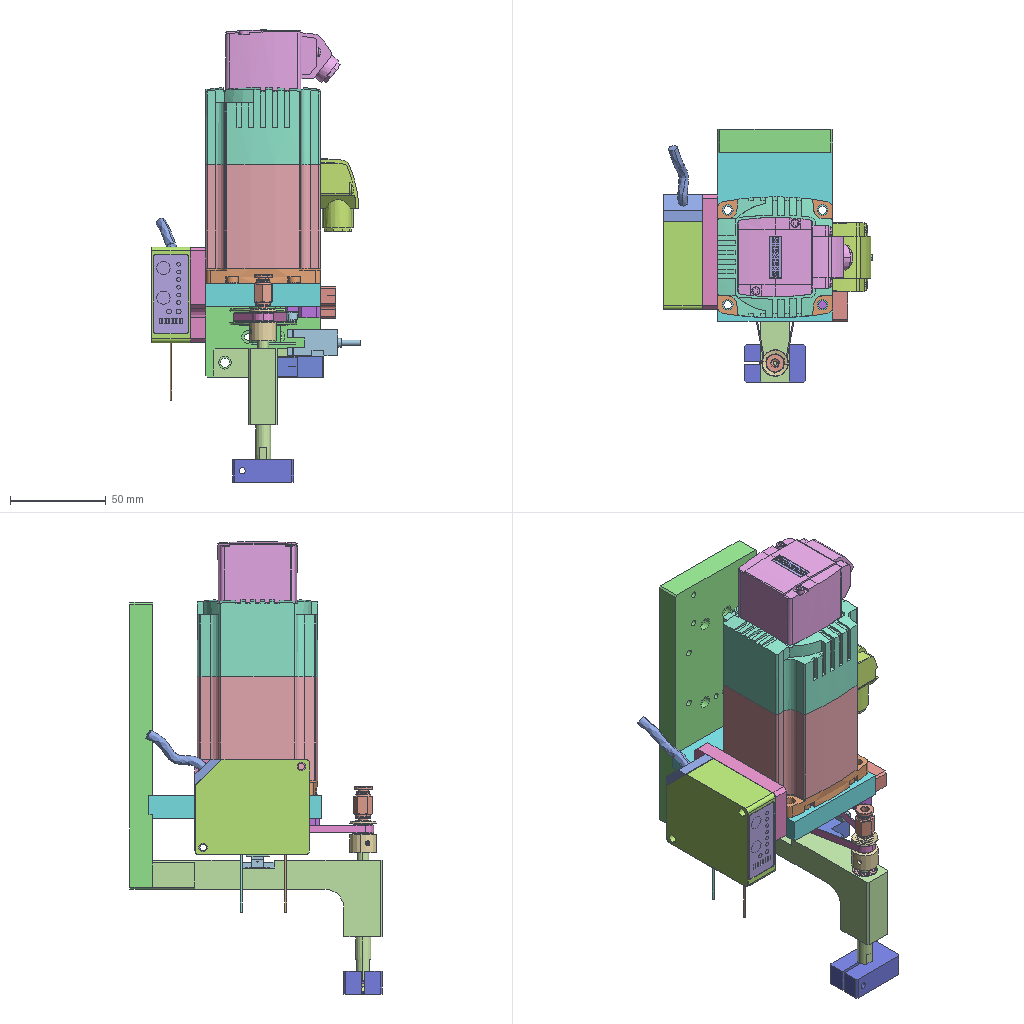Assembly | SolidWorks | 30 different items | 33 placed | box 109 x 132 x 237 mm
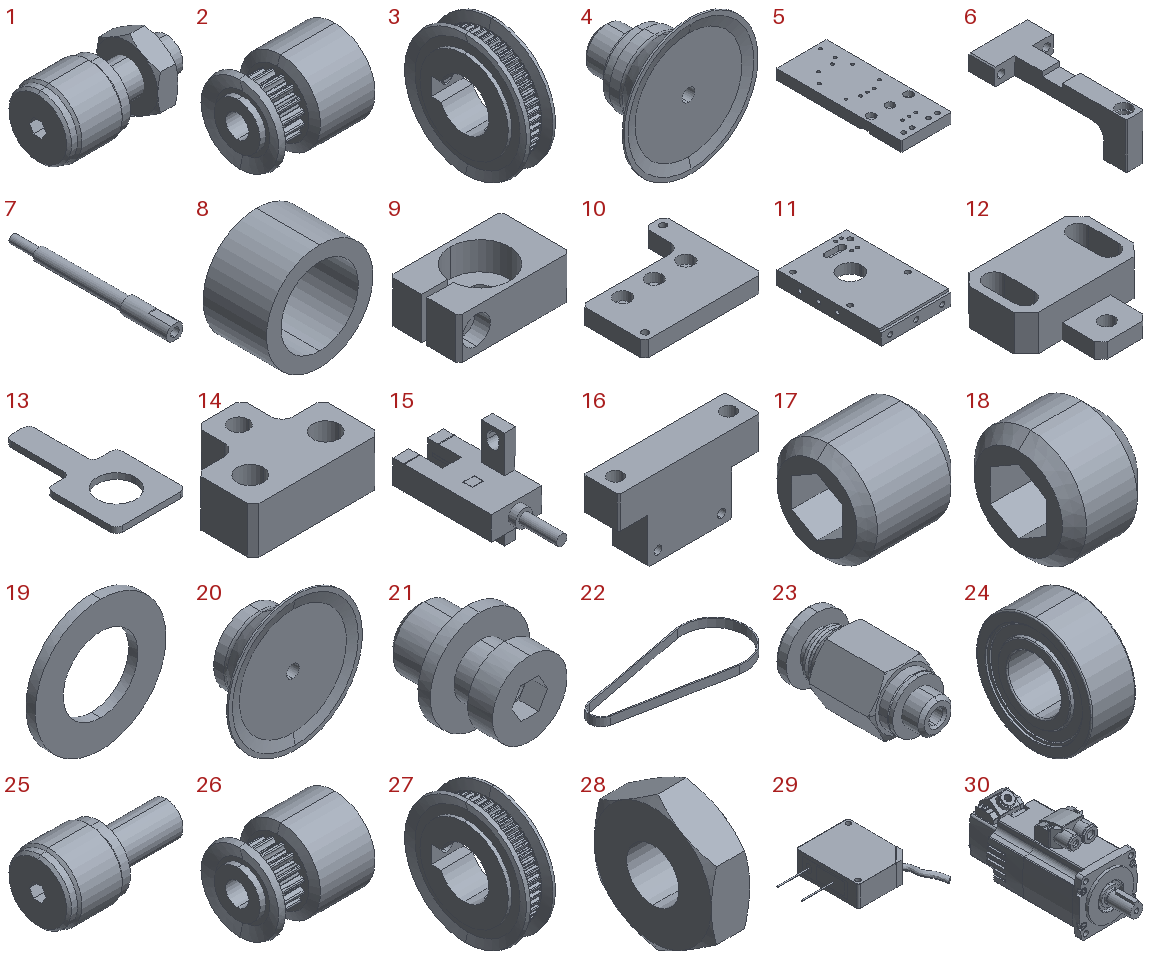Parts list (item | name | quantity | parent item | size | volume | features):
1 | (subassembly) | x1 | - | 11.5 x 6 x 6.351 mm | 226.743 mm3 | -
2 | (subassembly) | x1 | - | 17 x 14 x 14 mm | 1805 mm3 | -
3 | (subassembly) | x1 | - | 9 x 35 x 35 mm | 4712 mm3 | -
4 | (subassembly) | x1 | - | 16 x 10.5 x 16 mm | 558.242 mm3 | features AEMSimFeature 1
5 | - | x1 | - | 60 x 150 x 12 mm | 102302 mm3 | features HoleWzd 8, ICE 2, Chamfer 1, Extrusion 1, LPattern 1
6 | - | x1 | - | 52 x 120 x 40 mm | 40575 mm3 | features ICE 10, HoleWzd 3, Chamfer 1, Extrusion 1, Fillet 1, MirrorPattern 1
7 | - | x1 | - | 8 x 80 x 8 mm | 2165 mm3 | features ICE 4, HoleWzd 1, Revolution 1
8 | - | x1 | - | 8.4 x 5 x 8.4 mm | 130.965 mm3 | features Revolution 1
9 | - | x1 | - | 32 x 20 x 12 mm | 5110 mm3 | features ICE 3, HoleWzd 2, Chamfer 1, Extrusion 1, RevCut 1
10 | - | x1 | - | 60 x 50 x 8 mm | 15791 mm3 | features Chamfer 2, HoleWzd 2, Extrusion 1, Fillet 1, ICE 1
11 | - | x1 | - | 60 x 90 x 12 mm | 52743 mm3 | features HoleWzd 7, ICE 5, Chamfer 1, Cut 1, Extrusion 1, MoveFace 1
12 | - | x1 | - | 20 x 18 x 6 mm | 1134 mm3 | features HoleWzd 3, Chamfer 2, ICE 2, Extrusion 1
13 | - | x1 | - | 12 x 23 x 1 mm | 152.93 mm3 | features Extrusion 1, Fillet 1, HoleWzd 1
14 | - | x1 | - | 22 x 17 x 8 mm | 1559 mm3 | features HoleWzd 2, Chamfer 1, Extrusion 1, Fillet 1, ICE 1
15 | - | x1 | - | 13.7 x 38.4 x 26 mm | 2302 mm3 | features BaseBody 1
16 | - | x1 | - | 44 x 11 x 24 mm | 8094 mm3 | features Chamfer 2, HoleWzd 2, Extrusion 1, ICE 1
17 | - | x2 | in 2 | 3 x 3 x 3 mm | 17.153 mm3 | features BaseBody 1
18 | - | x2 | in 3 | 3 x 4 x 4 mm | 27.73 mm3 | features BaseBody 1
19 | - | x1 | in 4 | 7 x 0.5 x 7 mm | 12.959 mm3 | features BaseBody 1
20 | - | x1 | in 4 | 16 x 5.5 x 16 mm | 386.03 mm3 | features BaseBody 1
21 | - | x1 | in 4 | 8 x 9 x 8 mm | 159.238 mm3 | features BaseBody 1
22 | - | x1 | - | 76.775 x 31.76 x 4 mm | 427.631 mm3 | features Extrusion 1
23 | - | x1 | - | 10.392 x 19.5 x 9.5 mm | 848.774 mm3 | features BaseBody 1
24 | - | x2 | - | 5 x 13 x 13 mm | 402.825 mm3 | features BaseBody 1
25 | - | x1 | in 1 | 11.5 x 6 x 6 mm | 188.495 mm3 | features BaseBody 1
26 | - | x1 | in 2 | 17 x 14 x 14 mm | 1770 mm3 | features BaseBody 1
27 | - | x1 | in 3 | 9 x 35 x 35 mm | 4657 mm3 | features BaseBody 1
28 | - | x1 | in 1 | 1.8 x 5.5 x 6.351 mm | 38.246 mm3 | features BaseBody 1
29 | - | x1 | - | 95.223 x 85.573 x 20.4 mm | 60474 mm3 | features BaseBody 6
30 | - | x1 | - | 63.062 x 163.688 x 80 mm | 352083 mm3 | features BaseBody 8
Mates (type | each side: item.copy, entity, surface, feature):
Concentric | 7.1 face cylinder Revolve1 | 24.1 face cylinder Input1
Coincident | 8.1 face plane Revolve1 | 24.1 face plane Input1
Coincident | 24.1 face plane Input1 | 6.1 face plane Cut-Extrude6
Concentric | 7.1 face cylinder Revolve1 | 24.2 face cylinder Input1
Coincident | 7.1 face plane Revolve1 | 24.2 face plane Input1
Coincident | 24.2 face plane Input1 | 6.1 face plane Cut-Extrude7
Coincident | 29.1 face plane Input2 | 10.1 face plane Boss-Extrude1
Concentric | 29.1 face cylinder Input2 | 10.1 face cylinder M4 Tapped Hole1 | 2 times
Coincident | 5.1 face plane Boss-Extrude1 | 6.1 face plane Boss-Extrude1 | 2 times
Width | 6.1 face plane Boss-Extrude1 | 6.1 face plane Boss-Extrude1 | 5.1 face plane Boss-Extrude1 | 5.1 face plane Boss-Extrude1 | 2 times
Coincident | 5.1 face plane Cut-Extrude2 | 11.1 face plane Boss-Extrude1
Concentric | 5.1 face cylinder CBORE for M5 Hex Socket Head Cap Screw1 | 11.1 face cylinder M5 Tapped Hole1 | 2 times
Concentric | 7.1 face cylinder Revolve1 | 8.1 face cylinder Revolve1
Coincident | 15.1 face plane Input1 | 16.1 face plane Boss-Extrude1
Slot | 15.1 face plane Input1 | 16.1 face cylinder M3 Tapped Hole1 | 2 times
Concentric | 7.1 face cylinder M5x0.75 Tapped Hole1 | 21.1 face cylinder ZP2A-M02P_MT
Coincident | 7.1 face plane Revolve1 | 19.1 face plane ZP-5G2_MT
Coincident | 9.1 face plane Boss-Extrude1 | 20.1 face plane ZP2-B15MTS_PAD
Concentric | 7.1 face cylinder Revolve1 | 9.1 edge
Parallel | 6.1 face plane Boss-Extrude1 | 9.1 face plane Boss-Extrude1
Concentric | 7.1 face cylinder Revolve1 | 6.1 face cylinder Cut-Extrude7
Width | 22.1 face plane Boss-Extrude1 | 22.1 face plane Boss-Extrude1 | 6.1 face plane Mirror1 | 6.1 face plane Cut-Extrude4
Coincident | 6.1 face plane Mirror1 | 16.1 face plane Boss-Extrude1
Coincident | 6.1 face plane Cut-Extrude8 | 16.1 face plane Boss-Extrude1
Width | 16.1 face plane Boss-Extrude1 | 16.1 face plane Boss-Extrude1 | 6.1 face plane Cut-Extrude8 | 6.1 face plane Cut-Extrude8
Coincident | 10.1 face plane Boss-Extrude1 | 11.1 face plane Boss-Extrude1
Concentric | 10.1 face cylinder CBORE for M4 Hex Socket Head Cap Screw1 | 11.1 face cylinder M4 Tapped Hole2
Parallel | 10.1 face plane Cut-Extrude1 | 11.1 face plane Boss-Extrude1
Coincident | 11.1 face plane Boss-Extrude1 | 30.1 face plane 1_7-1-solid1
Parallel | 11.1 face plane Boss-Extrude1 | 27.1 face plane Input1
DistanceDim | 11.1 face plane Boss-Extrude1 | 27.1 face plane Input1
Concentric | 11.1 face cylinder M5 Tapped Hole2 | 30.1 face cylinder 1_7-1-solid1 | 2 times
DistanceDim | 25.1 face plane Input1 | 11.1 face plane Boss-Extrude1
Coincident | 11.1 face plane Boss-Extrude1 | 14.1 face plane Boss-Extrude1
Concentric | 11.1 face cylinder M3 Tapped Hole2 | 12.1 face cylinder M3 Clearance Slot1 | 2 times
Concentric | 11.1 face cylinder M4 Tapped Hole3 | 14.1 face cylinder CBORE for M4 Hexagon socket head cap screws1 | 2 times
Concentric | 7.1 face cylinder Revolve1 | 26.1 face cylinder Input1
Coincident | 26.1 face plane Input1 | 27.1 face plane Input1
Concentric | 26.1 face cylinder Input1 | 22.1 face cylinder Boss-Extrude1
Concentric | 30.1 face cylinder 1-1-solid1 | 27.1 face cylinder Input1
Coincident | 30.1 face plane 1-1-solid1 | 13.1 face plane Boss-Extrude1
Concentric | 30.1 face cylinder 1-1-solid1 | 13.1 face cylinder M6 Clearance Hole1
Concentric | 25.1 face cylinder Input1 | 12.1 face cylinder M3 Tapped Hole1
Coincident | 25.1 face plane Input1 | 12.1 face plane Cut-Extrude1